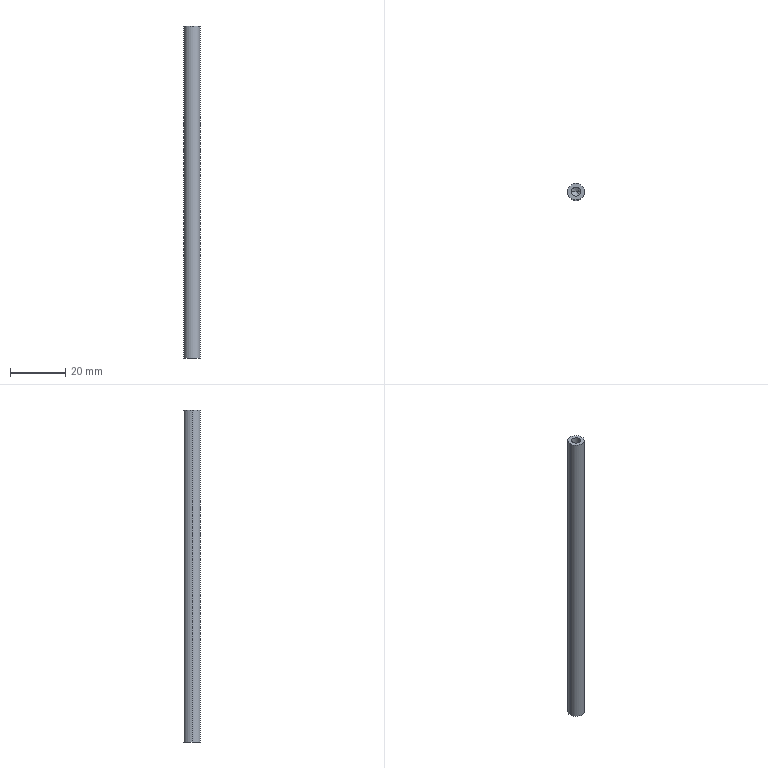Part | SolidWorks | features HoleWzd 2, Extrusion 1 | 1 solid | 12 faces | box 6 x 6 x 120 mm | volume 3214 mm3 | cylinder 6 | cone 4 | plane 2 | commonest cylinder face diameters 3.3 x4 6 x2
STEP:
#1=CARTESIAN_POINT('',(1.65,0.,-49.9));
#2=VERTEX_POINT('',#1);
#3=CARTESIAN_POINT('',(-1.65,0.,-49.9));
#4=VERTEX_POINT('',#3);
#5=CARTESIAN_POINT('',(0.,0.,-49.9));
#6=DIRECTION('',(0.,0.,-1.));
#7=DIRECTION('',(-1.,0.,0.));
#8=AXIS2_PLACEMENT_3D('',#5,#6,#7);
#9=CIRCLE('',#8,1.65);
#10=EDGE_CURVE('',#2,#4,#9,.T.);
#11=ORIENTED_EDGE('',*,*,#10,.F.);
#12=CARTESIAN_POINT('',(1.65,0.,-60.));
#13=VERTEX_POINT('',#12);
#14=CARTESIAN_POINT('',(1.65,0.,-60.));
#15=DIRECTION('',(0.,0.,-1.));
#16=VECTOR('',#15,1000.);
#17=LINE('',#14,#16);
#18=EDGE_CURVE('',#2,#13,#17,.T.);
#19=ORIENTED_EDGE('',*,*,#18,.T.);
#20=CARTESIAN_POINT('',(-1.65,0.,-60.));
#21=VERTEX_POINT('',#20);
#22=CARTESIAN_POINT('',(0.,0.,-60.));
#23=DIRECTION('',(0.,0.,-1.));
#24=DIRECTION('',(-1.,0.,0.));
#25=AXIS2_PLACEMENT_3D('',#22,#23,#24);
#26=CIRCLE('',#25,1.65);
#27=EDGE_CURVE('',#13,#21,#26,.T.);
#28=ORIENTED_EDGE('',*,*,#27,.T.);
#29=CARTESIAN_POINT('',(-1.65,0.,-60.));
#30=DIRECTION('',(0.,0.,-1.));
#31=VECTOR('',#30,1000.);
#32=LINE('',#29,#31);
#33=EDGE_CURVE('',#4,#21,#32,.T.);
#34=ORIENTED_EDGE('',*,*,#33,.F.);
#35=EDGE_LOOP('',(#11,#19,#28,#34));
#36=FACE_OUTER_BOUND('',#35,.T.);
#37=CARTESIAN_POINT('',(0.,0.,-60.));
#38=DIRECTION('',(0.,0.,-1.));
#39=DIRECTION('',(-1.,0.,0.));
#40=AXIS2_PLACEMENT_3D('',#37,#38,#39);
#41=CYLINDRICAL_SURFACE('',#40,1.65);
#42=ADVANCED_FACE('',(#36),#41,.F.);
#43=CARTESIAN_POINT('',(0.,0.,-48.909));
#44=VERTEX_POINT('',#43);
#45=CARTESIAN_POINT('',(-1.65,0.,-49.9));
#46=DIRECTION('',(-0.8572,0.,-0.515));
#47=VECTOR('',#46,1000.);
#48=LINE('',#45,#47);
#49=EDGE_CURVE('',#44,#4,#48,.T.);
#50=ORIENTED_EDGE('',*,*,#49,.F.);
#51=CARTESIAN_POINT('',(1.65,0.,-49.9));
#52=DIRECTION('',(0.8572,0.,-0.515));
#53=VECTOR('',#52,1000.);
#54=LINE('',#51,#53);
#55=EDGE_CURVE('',#44,#2,#54,.T.);
#56=ORIENTED_EDGE('',*,*,#55,.T.);
#57=ORIENTED_EDGE('',*,*,#10,.T.);
#58=EDGE_LOOP('',(#50,#56,#57));
#59=FACE_OUTER_BOUND('',#58,.T.);
#60=CARTESIAN_POINT('',(0.,0.,-49.9));
#61=DIRECTION('',(0.,0.,-1.));
#62=DIRECTION('',(-1.,0.,0.));
#63=AXIS2_PLACEMENT_3D('',#60,#61,#62);
#64=CONICAL_SURFACE('',#63,1.65,1.03);
#65=ADVANCED_FACE('',(#59),#64,.F.);
#66=CARTESIAN_POINT('',(-1.65,0.,49.9));
#67=VERTEX_POINT('',#66);
#68=CARTESIAN_POINT('',(1.65,0.,49.9));
#69=VERTEX_POINT('',#68);
#70=CARTESIAN_POINT('',(0.,0.,49.9));
#71=DIRECTION('',(0.,0.,1.));
#72=DIRECTION('',(1.,0.,0.));
#73=AXIS2_PLACEMENT_3D('',#70,#71,#72);
#74=CIRCLE('',#73,1.65);
#75=EDGE_CURVE('',#67,#69,#74,.T.);
#76=ORIENTED_EDGE('',*,*,#75,.F.);
#77=CARTESIAN_POINT('',(-1.65,0.,60.));
#78=VERTEX_POINT('',#77);
#79=CARTESIAN_POINT('',(-1.65,0.,60.));
#80=DIRECTION('',(0.,0.,1.));
#81=VECTOR('',#80,1000.);
#82=LINE('',#79,#81);
#83=EDGE_CURVE('',#67,#78,#82,.T.);
#84=ORIENTED_EDGE('',*,*,#83,.T.);
#85=CARTESIAN_POINT('',(1.65,0.,60.));
#86=VERTEX_POINT('',#85);
#87=CARTESIAN_POINT('',(0.,0.,60.));
#88=DIRECTION('',(0.,0.,1.));
#89=DIRECTION('',(1.,0.,0.));
#90=AXIS2_PLACEMENT_3D('',#87,#88,#89);
#91=CIRCLE('',#90,1.65);
#92=EDGE_CURVE('',#78,#86,#91,.T.);
#93=ORIENTED_EDGE('',*,*,#92,.T.);
#94=CARTESIAN_POINT('',(1.65,0.,60.));
#95=DIRECTION('',(0.,0.,1.));
#96=VECTOR('',#95,1000.);
#97=LINE('',#94,#96);
#98=EDGE_CURVE('',#69,#86,#97,.T.);
#99=ORIENTED_EDGE('',*,*,#98,.F.);
#100=EDGE_LOOP('',(#76,#84,#93,#99));
#101=FACE_OUTER_BOUND('',#100,.T.);
#102=CARTESIAN_POINT('',(0.,0.,60.));
#103=DIRECTION('',(0.,0.,1.));
#104=DIRECTION('',(1.,0.,0.));
#105=AXIS2_PLACEMENT_3D('',#102,#103,#104);
#106=CYLINDRICAL_SURFACE('',#105,1.65);
#107=ADVANCED_FACE('',(#101),#106,.F.);
#108=CARTESIAN_POINT('',(0.,0.,48.909));
#109=VERTEX_POINT('',#108);
#110=CARTESIAN_POINT('',(1.65,0.,49.9));
#111=DIRECTION('',(0.8572,0.,0.515));
#112=VECTOR('',#111,1000.);
#113=LINE('',#110,#112);
#114=EDGE_CURVE('',#109,#69,#113,.T.);
#115=ORIENTED_EDGE('',*,*,#114,.F.);
#116=CARTESIAN_POINT('',(-1.65,0.,49.9));
#117=DIRECTION('',(-0.8572,0.,0.515));
#118=VECTOR('',#117,1000.);
#119=LINE('',#116,#118);
#120=EDGE_CURVE('',#109,#67,#119,.T.);
#121=ORIENTED_EDGE('',*,*,#120,.T.);
#122=ORIENTED_EDGE('',*,*,#75,.T.);
#123=EDGE_LOOP('',(#115,#121,#122));
#124=FACE_OUTER_BOUND('',#123,.T.);
#125=CARTESIAN_POINT('',(0.,0.,49.9));
#126=DIRECTION('',(0.,0.,1.));
#127=DIRECTION('',(1.,0.,0.));
#128=AXIS2_PLACEMENT_3D('',#125,#126,#127);
#129=CONICAL_SURFACE('',#128,1.65,1.03);
#130=ADVANCED_FACE('',(#124),#129,.F.);
#131=CARTESIAN_POINT('',(3.,0.,60.));
#132=VERTEX_POINT('',#131);
#133=CARTESIAN_POINT('',(-3.,0.,60.));
#134=VERTEX_POINT('',#133);
#135=CARTESIAN_POINT('',(0.,0.,60.));
#136=DIRECTION('',(0.,0.,1.));
#137=DIRECTION('',(1.,0.,0.));
#138=AXIS2_PLACEMENT_3D('',#135,#136,#137);
#139=CIRCLE('',#138,3.);
#140=EDGE_CURVE('',#132,#134,#139,.T.);
#141=ORIENTED_EDGE('',*,*,#140,.F.);
#142=CARTESIAN_POINT('',(3.,0.,-60.));
#143=VERTEX_POINT('',#142);
#144=CARTESIAN_POINT('',(3.,0.,60.));
#145=DIRECTION('',(0.,0.,-1.));
#146=VECTOR('',#145,1000.);
#147=LINE('',#144,#146);
#148=EDGE_CURVE('',#132,#143,#147,.T.);
#149=ORIENTED_EDGE('',*,*,#148,.T.);
#150=CARTESIAN_POINT('',(-3.,0.,-60.));
#151=VERTEX_POINT('',#150);
#152=CARTESIAN_POINT('',(0.,0.,-60.));
#153=DIRECTION('',(0.,0.,1.));
#154=DIRECTION('',(1.,0.,0.));
#155=AXIS2_PLACEMENT_3D('',#152,#153,#154);
#156=CIRCLE('',#155,3.);
#157=EDGE_CURVE('',#143,#151,#156,.T.);
#158=ORIENTED_EDGE('',*,*,#157,.T.);
#159=CARTESIAN_POINT('',(-3.,0.,60.));
#160=DIRECTION('',(0.,0.,-1.));
#161=VECTOR('',#160,1000.);
#162=LINE('',#159,#161);
#163=EDGE_CURVE('',#134,#151,#162,.T.);
#164=ORIENTED_EDGE('',*,*,#163,.F.);
#165=EDGE_LOOP('',(#141,#149,#158,#164));
#166=FACE_OUTER_BOUND('',#165,.T.);
#167=CARTESIAN_POINT('',(0.,0.,60.));
#168=DIRECTION('',(0.,0.,-1.));
#169=DIRECTION('',(-1.,0.,0.));
#170=AXIS2_PLACEMENT_3D('',#167,#168,#169);
#171=CYLINDRICAL_SURFACE('',#170,3.);
#172=ADVANCED_FACE('',(#166),#171,.T.);
#173=ORIENTED_EDGE('',*,*,#148,.F.);
#174=CARTESIAN_POINT('',(0.,0.,60.));
#175=DIRECTION('',(0.,0.,1.));
#176=DIRECTION('',(1.,0.,0.));
#177=AXIS2_PLACEMENT_3D('',#174,#175,#176);
#178=CIRCLE('',#177,3.);
#179=EDGE_CURVE('',#134,#132,#178,.T.);
#180=ORIENTED_EDGE('',*,*,#179,.F.);
#181=ORIENTED_EDGE('',*,*,#163,.T.);
#182=CARTESIAN_POINT('',(0.,0.,-60.));
#183=DIRECTION('',(0.,0.,1.));
#184=DIRECTION('',(1.,0.,0.));
#185=AXIS2_PLACEMENT_3D('',#182,#183,#184);
#186=CIRCLE('',#185,3.);
#187=EDGE_CURVE('',#151,#143,#186,.T.);
#188=ORIENTED_EDGE('',*,*,#187,.T.);
#189=EDGE_LOOP('',(#173,#180,#181,#188));
#190=FACE_OUTER_BOUND('',#189,.T.);
#191=CARTESIAN_POINT('',(0.,0.,60.));
#192=DIRECTION('',(0.,0.,-1.));
#193=DIRECTION('',(-1.,0.,0.));
#194=AXIS2_PLACEMENT_3D('',#191,#192,#193);
#195=CYLINDRICAL_SURFACE('',#194,3.);
#196=ADVANCED_FACE('',(#190),#195,.T.);
#197=CARTESIAN_POINT('',(0.,0.,60.));
#198=DIRECTION('',(0.,0.,1.));
#199=DIRECTION('',(1.,0.,0.));
#200=AXIS2_PLACEMENT_3D('',#197,#198,#199);
#201=CIRCLE('',#200,1.65);
#202=EDGE_CURVE('',#86,#78,#201,.T.);
#203=ORIENTED_EDGE('',*,*,#202,.F.);
#204=ORIENTED_EDGE('',*,*,#92,.F.);
#205=EDGE_LOOP('',(#203,#204));
#206=FACE_BOUND('',#205,.T.);
#207=ORIENTED_EDGE('',*,*,#179,.T.);
#208=ORIENTED_EDGE('',*,*,#140,.T.);
#209=EDGE_LOOP('',(#207,#208));
#210=FACE_OUTER_BOUND('',#209,.T.);
#211=CARTESIAN_POINT('',(0.,0.,60.));
#212=DIRECTION('',(0.,0.,1.));
#213=DIRECTION('',(1.,0.,0.));
#214=AXIS2_PLACEMENT_3D('',#211,#212,#213);
#215=PLANE('',#214);
#216=ADVANCED_FACE('',(#206,#210),#215,.T.);
#217=CARTESIAN_POINT('',(0.,0.,-60.));
#218=DIRECTION('',(0.,0.,-1.));
#219=DIRECTION('',(-1.,0.,0.));
#220=AXIS2_PLACEMENT_3D('',#217,#218,#219);
#221=CIRCLE('',#220,1.65);
#222=EDGE_CURVE('',#21,#13,#221,.T.);
#223=ORIENTED_EDGE('',*,*,#222,.F.);
#224=ORIENTED_EDGE('',*,*,#27,.F.);
#225=EDGE_LOOP('',(#223,#224));
#226=FACE_BOUND('',#225,.T.);
#227=ORIENTED_EDGE('',*,*,#187,.F.);
#228=ORIENTED_EDGE('',*,*,#157,.F.);
#229=EDGE_LOOP('',(#227,#228));
#230=FACE_OUTER_BOUND('',#229,.T.);
#231=CARTESIAN_POINT('',(0.,0.,-60.));
#232=DIRECTION('',(0.,0.,1.));
#233=DIRECTION('',(1.,0.,0.));
#234=AXIS2_PLACEMENT_3D('',#231,#232,#233);
#235=PLANE('',#234);
#236=ADVANCED_FACE('',(#226,#230),#235,.F.);
#237=ORIENTED_EDGE('',*,*,#120,.F.);
#238=ORIENTED_EDGE('',*,*,#114,.T.);
#239=CARTESIAN_POINT('',(0.,0.,49.9));
#240=DIRECTION('',(0.,0.,1.));
#241=DIRECTION('',(1.,0.,0.));
#242=AXIS2_PLACEMENT_3D('',#239,#240,#241);
#243=CIRCLE('',#242,1.65);
#244=EDGE_CURVE('',#69,#67,#243,.T.);
#245=ORIENTED_EDGE('',*,*,#244,.T.);
#246=EDGE_LOOP('',(#237,#238,#245));
#247=FACE_OUTER_BOUND('',#246,.T.);
#248=CARTESIAN_POINT('',(0.,0.,49.9));
#249=DIRECTION('',(0.,0.,1.));
#250=DIRECTION('',(1.,0.,0.));
#251=AXIS2_PLACEMENT_3D('',#248,#249,#250);
#252=CONICAL_SURFACE('',#251,1.65,1.03);
#253=ADVANCED_FACE('',(#247),#252,.F.);
#254=ORIENTED_EDGE('',*,*,#83,.F.);
#255=ORIENTED_EDGE('',*,*,#244,.F.);
#256=ORIENTED_EDGE('',*,*,#98,.T.);
#257=ORIENTED_EDGE('',*,*,#202,.T.);
#258=EDGE_LOOP('',(#254,#255,#256,#257));
#259=FACE_OUTER_BOUND('',#258,.T.);
#260=CARTESIAN_POINT('',(0.,0.,60.));
#261=DIRECTION('',(0.,0.,1.));
#262=DIRECTION('',(1.,0.,0.));
#263=AXIS2_PLACEMENT_3D('',#260,#261,#262);
#264=CYLINDRICAL_SURFACE('',#263,1.65);
#265=ADVANCED_FACE('',(#259),#264,.F.);
#266=ORIENTED_EDGE('',*,*,#55,.F.);
#267=ORIENTED_EDGE('',*,*,#49,.T.);
#268=CARTESIAN_POINT('',(0.,0.,-49.9));
#269=DIRECTION('',(0.,0.,-1.));
#270=DIRECTION('',(-1.,0.,0.));
#271=AXIS2_PLACEMENT_3D('',#268,#269,#270);
#272=CIRCLE('',#271,1.65);
#273=EDGE_CURVE('',#4,#2,#272,.T.);
#274=ORIENTED_EDGE('',*,*,#273,.T.);
#275=EDGE_LOOP('',(#266,#267,#274));
#276=FACE_OUTER_BOUND('',#275,.T.);
#277=CARTESIAN_POINT('',(0.,0.,-49.9));
#278=DIRECTION('',(0.,0.,-1.));
#279=DIRECTION('',(-1.,0.,0.));
#280=AXIS2_PLACEMENT_3D('',#277,#278,#279);
#281=CONICAL_SURFACE('',#280,1.65,1.03);
#282=ADVANCED_FACE('',(#276),#281,.F.);
#283=ORIENTED_EDGE('',*,*,#18,.F.);
#284=ORIENTED_EDGE('',*,*,#273,.F.);
#285=ORIENTED_EDGE('',*,*,#33,.T.);
#286=ORIENTED_EDGE('',*,*,#222,.T.);
#287=EDGE_LOOP('',(#283,#284,#285,#286));
#288=FACE_OUTER_BOUND('',#287,.T.);
#289=CARTESIAN_POINT('',(0.,0.,-60.));
#290=DIRECTION('',(0.,0.,-1.));
#291=DIRECTION('',(-1.,0.,0.));
#292=AXIS2_PLACEMENT_3D('',#289,#290,#291);
#293=CYLINDRICAL_SURFACE('',#292,1.65);
#294=ADVANCED_FACE('',(#288),#293,.F.);
#295=CLOSED_SHELL('',(#42,#65,#107,#130,#172,#196,#216,#236,#253,#265,#282,#294));
#296=MANIFOLD_SOLID_BREP('',#295);
#297=CARTESIAN_POINT('',(0.,0.,0.));
#298=DIRECTION('',(0.,0.,1.));
#299=DIRECTION('',(1.,0.,0.));
#300=AXIS2_PLACEMENT_3D('',#297,#298,#299);
#301=(LENGTH_UNIT()NAMED_UNIT(*)SI_UNIT(.MILLI.,.METRE.));
#302=UNCERTAINTY_MEASURE_WITH_UNIT(LENGTH_MEASURE(0.00001),#301,'','');
#303=(NAMED_UNIT(*)PLANE_ANGLE_UNIT()SI_UNIT($,.RADIAN.));
#304=(NAMED_UNIT(*)SI_UNIT($,.STERADIAN.)SOLID_ANGLE_UNIT());
#305=(GEOMETRIC_REPRESENTATION_CONTEXT(3)GLOBAL_UNCERTAINTY_ASSIGNED_CONTEXT((#302))GLOBAL_UNIT_ASSIGNED_CONTEXT((#301,#303,#304))REPRESENTATION_CONTEXT('',''));
#306=ADVANCED_BREP_SHAPE_REPRESENTATION('',(#296,#300),#305);